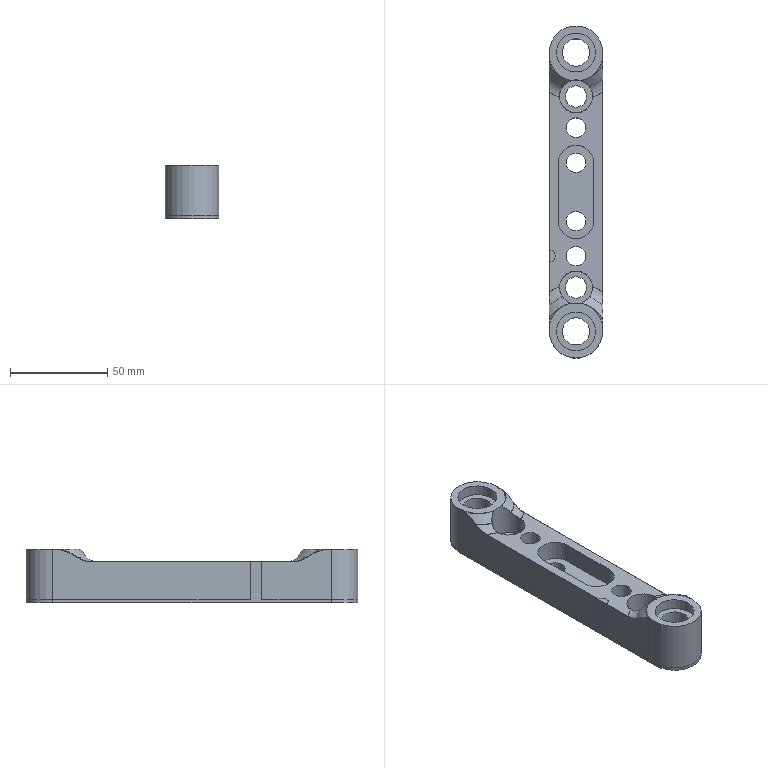NC program | NX | posted with a generic post | part box 27.4 x 170.48 x 27.5 mm
Lines 1 to 85 of 10888:
N10 G17 G21 G94 G90
(PLANAR_MILL , TOOL : D50R0.8)
N12 T01 M6
N14 G54
N16 G17 G0 G90 X120. Y0. B0. C0. S2000 M3
N18 G43 Z30. H1
N20 Z2.6
N22 G94 G1 Z0.6 F800.
N24 X90.
N26 X-90.
N28 X-120.
N30 Z2.6
N32 G0 Z30.
(PLANAR_MILL_COPY_1 , TOOL : D50R0.8)
N34 X120.
N36 Z2.3
N38 G1 Z0.3
N40 X90.
N42 X-90.
N44 X-120.
N46 Z2.3
N48 G0 Z30.
N50 M5
(DRILLING , TOOL : D8点钻)
N52 T02 M6
N54 G54
N56 G17 G0 G90 X-71.54 Y0. B0. C0. S2500 M3
N58 G43 Z30. H2
N60 G94 G81 G98 Z-1.5 F200. R3.
N62 X-49.
N64 X-33.
N66 X-15.
N68 X15.
N70 X33.
N72 X49.
N74 X71.54
N76 G80
N78 G0 X71.54 Y0. Z30.
N80 M5
(DRILLING_COPY , TOOL : D9.5钻头)
N82 T03 M6
N84 G54
N86 G17 G0 G90 X-33. Y0. B0. C0. S1600 M3
N88 G43 Z30. H3
N90 G94 G83 G98 Z-35. F150. Q2. R3.
N92 X33.
N94 G80
N96 G0 X33. Y0. Z30.
N98 M5
(DRILLING_COPY_COPY_1 , TOOL : Z8.5)
N100 T21 M6
N102 G54
N104 G17 G0 G90 X-15. Y0. B0. C0. S1600 M3
N106 G43 Z30. H21
N108 G94 G83 G98 Z-35. F150. Q2. R3.
N110 X15.
N112 G80
N114 G0 X15. Y0. Z30.
N116 M5
(DRILLING_COPY_COPY , TOOL : D11钻头)
N118 T04 M6
N120 G54
N122 G17 G0 G90 X71.54 Y0. B0. C0. S1600 M3
N124 G43 Z30. H4
N126 G94 G83 G98 Z-35. F150. Q2. R3.
N128 X49.
N130 X-49.
N132 X-71.54
N134 G80
N136 G0 X-71.54 Y0. Z30.
N138 M5